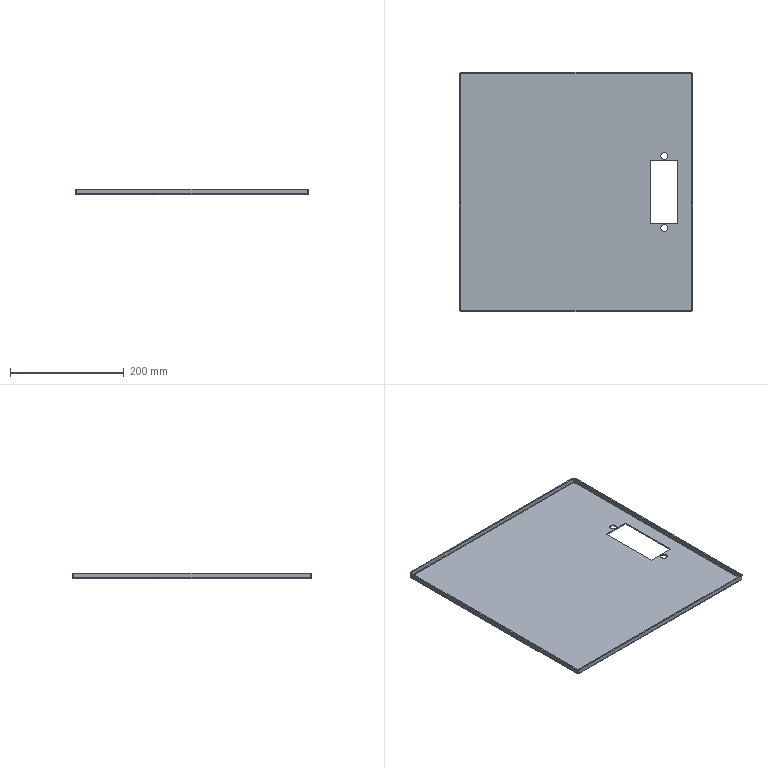Part | SolidWorks | features BaseBody 1 | 1 solid | 46 faces | box 410 x 420 x 10 mm | volume 356908 mm3 | plane 26 | cylinder 12 | spline 8 | commonest cylinder face diameters 1.473 x4 5.473 x4 12 x4